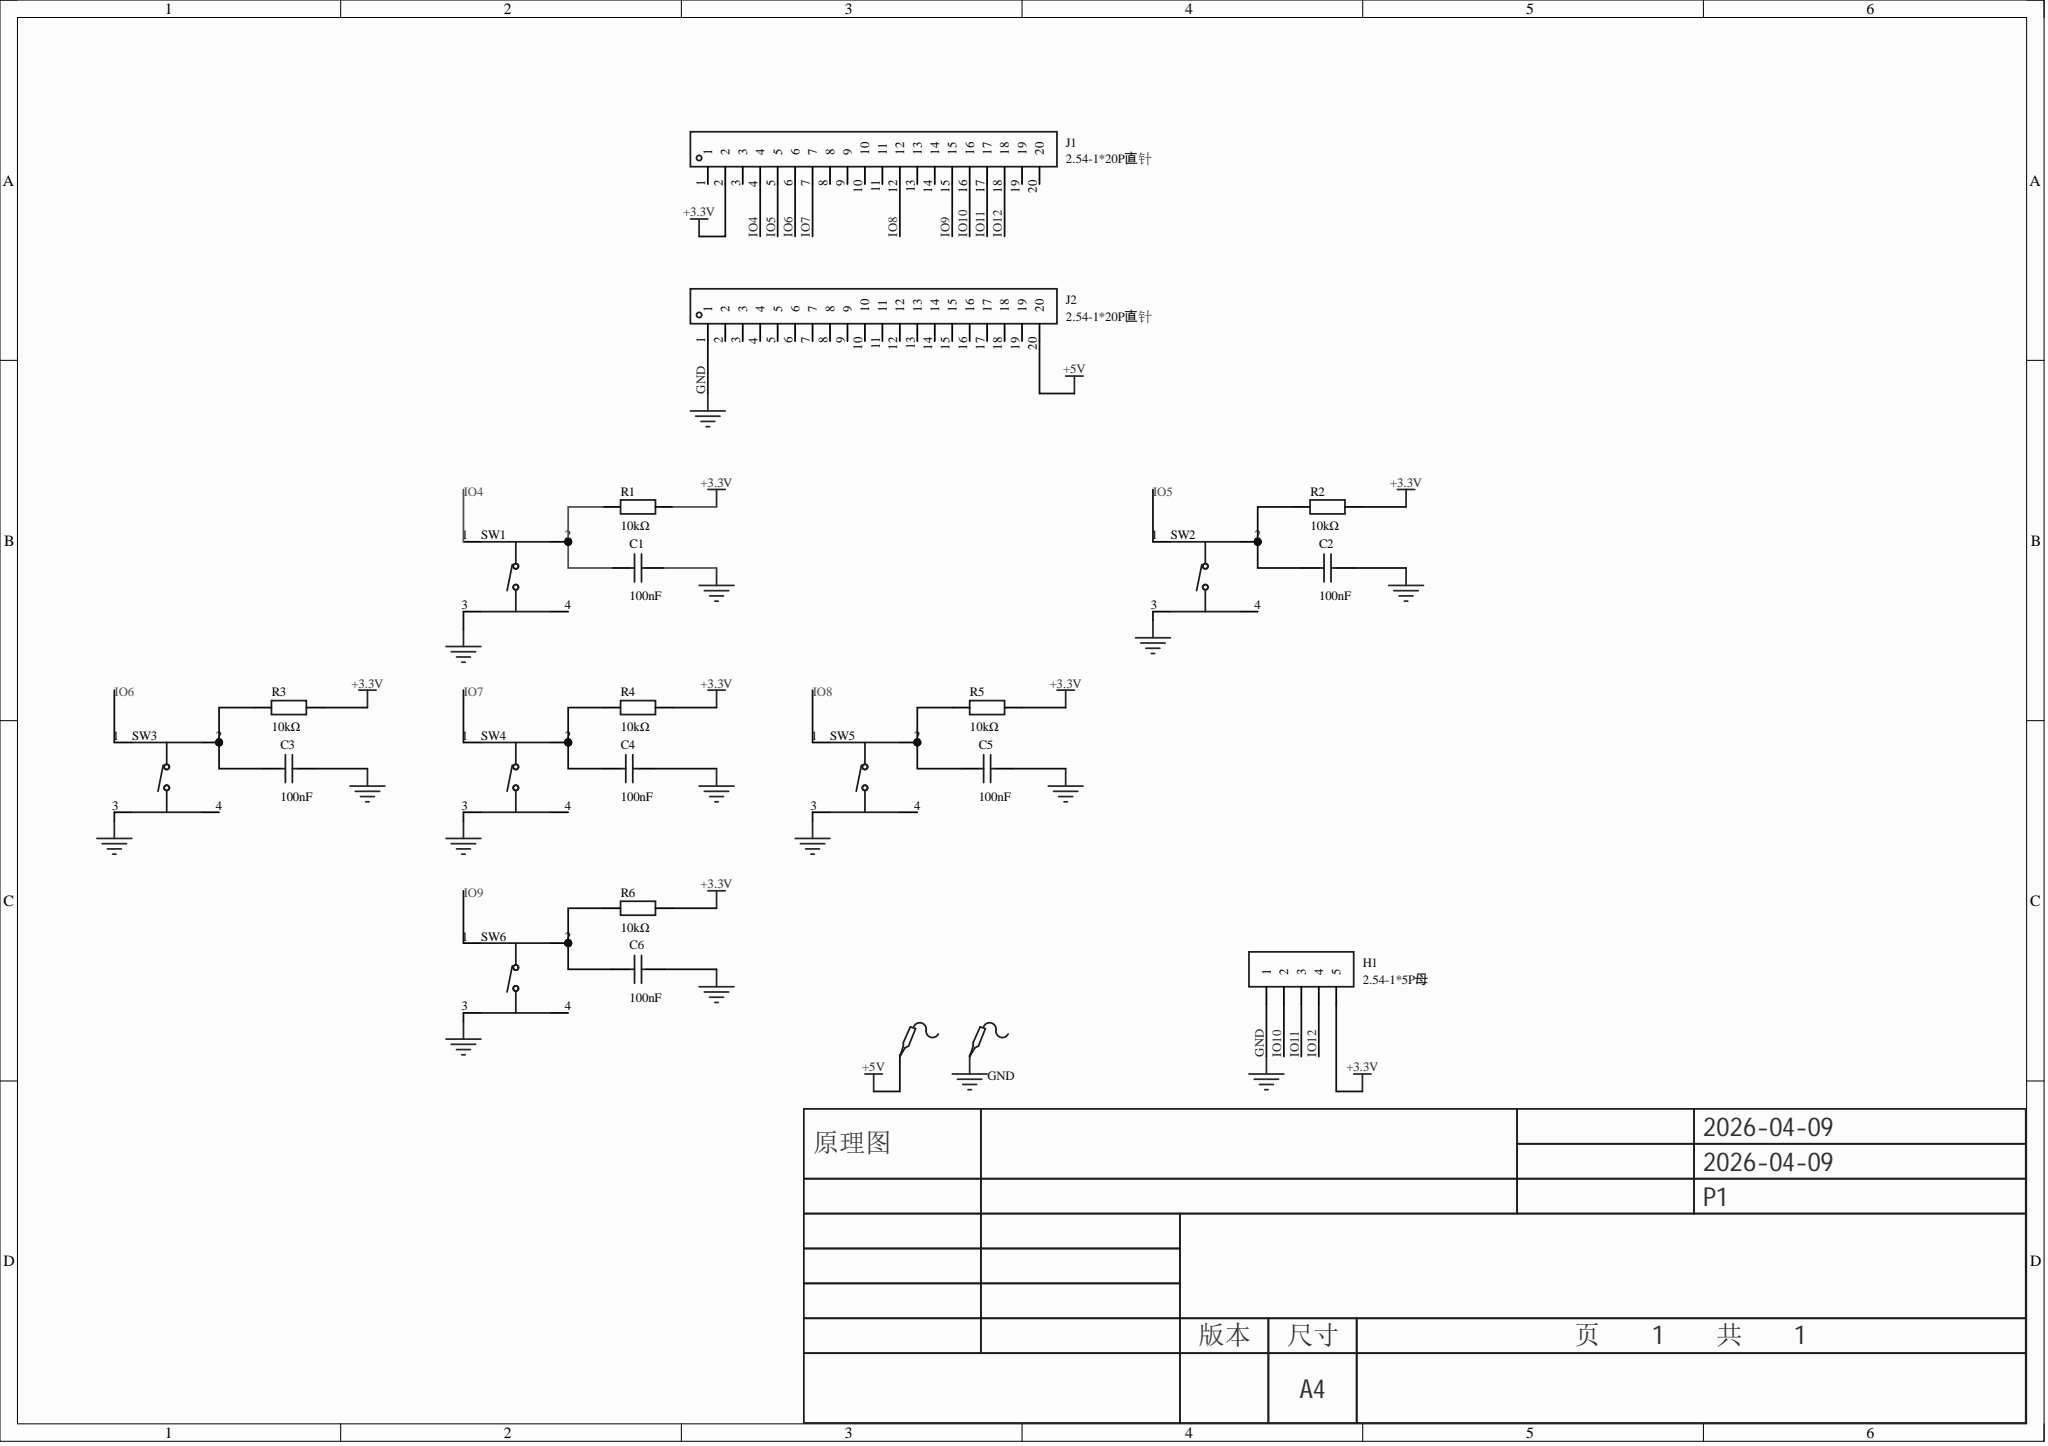Circuit board | Altium Designer | 23 parts | 18 nets
Bill of materials:
Comment,Description,Designator,Footprint,LibRef,Quantity
"","Test-Point","5V, GND","Test-Point-0.5mm","Test-Point","2"
"100nF","容值:100nF;精度:±10%;额定电压:100V;材质(温度系数):X7R;","C1, C2, C3, C4, C5, C6","C0805","CC0805KKX7R0BB104","6"
"2.54-1*5P母","间距:2.54mm;总孔位数:5;排数:1;插孔结构:1x5P;行距:-;安装类型:直插;塑高:-;触头材质:-;触头镀层:-;","H1","HDR-TH_5P-P2.54-V-F","2.54-1*5P母","1"
"2.54-1*20P直针","间距:2.54mm;总PIN位数:20;排数:1;插针结构:1x20P;行距:-;安装类型:直插;圆针/方针:方针;额定电流:3A;额定电压:-;配合针长度:-;塑高:-;端接针长度:-;触头材质:黄铜;触头镀层:-;工作温度范围:-40℃~+105℃;颜色:黑色;","J1, J2","HDR-TH_20P-P2.54-V-M-1","2.54-1*20P直针","2"
"10kΩ","","R1, R2, R3, R4, R5, R6","R0805","CR0805J80103G","6"
"TC-1103-C-K","","SW1, SW2, SW3, SW4, SW5, SW6","KEY-TH_4P-L12.0-W12.0-P5.00-LS12.5","TC-1103-C-K","6"
Netlist (Protel format):
[
5V
Test-Point-0.5mm




]
[
C1
C0805
100nF



]
[
C2
C0805
100nF



]
[
C3
C0805
100nF



]
[
C4
C0805
100nF



]
[
C5
C0805
100nF



]
[
C6
C0805
100nF



]
[
GND
Test-Point-0.5mm




]
[
H1
HDR-TH_5P-P2.54-V-F
2.54-1*5P母



]
[
J1
HDR-TH_20P-P2.54-V-M-1
2.54-1*20P直针



]
[
J2
HDR-TH_20P-P2.54-V-M-1
2.54-1*20P直针



]
[
R1
R0805
10kΩ



]
[
R2
R0805
10kΩ



]
[
R3
R0805
10kΩ



]
[
R4
R0805
10kΩ



]
[
R5
R0805
10kΩ



]
[
R6
R0805
10kΩ



]
[
SW1
KEY-TH_4P-L12.0-W12.0-P5.00-LS12.5
TC-1103-C-K



]
[
SW2
KEY-TH_4P-L12.0-W12.0-P5.00-LS12.5
TC-1103-C-K



]
[
SW3
KEY-TH_4P-L12.0-W12.0-P5.00-LS12.5
TC-1103-C-K



]
[
SW4
KEY-TH_4P-L12.0-W12.0-P5.00-LS12.5
TC-1103-C-K



]
[
SW5
KEY-TH_4P-L12.0-W12.0-P5.00-LS12.5
TC-1103-C-K



]
[
SW6
KEY-TH_4P-L12.0-W12.0-P5.00-LS12.5
TC-1103-C-K



]
(
NetC6_1
C6-1
R6-1
SW6-2
)
(
NetC5_1
C5-1
R5-1
SW5-2
)
(
NetC4_1
C4-1
R4-1
SW4-2
)
(
NetC3_1
C3-1
R3-1
SW3-2
)
(
NetC2_1
C2-1
R2-1
SW2-2
)
(
NetC1_1
C1-1
R1-1
SW1-2
)
(
IO12
H1-4
J1-18
)
(
IO11
H1-3
J1-17
)
(
IO10
H1-2
J1-16
)
(
IO9
J1-15
SW6-1
)
(
IO8
J1-12
SW5-1
)
(
IO7
J1-7
SW4-1
)
(
IO6
J1-6
SW3-1
)
(
IO5
J1-5
SW2-1
)
(
IO4
J1-4
SW1-1
)
(
GND
C1-2
C2-2
C3-2
C4-2
C5-2
C6-2
GND-1
H1-1
J2-1
SW1-3
SW2-3
SW3-3
SW4-3
SW5-3
SW6-3
)
(
+5V
5V-1
J2-20
)
(
+3.3V
H1-5
J1-2
R1-2
R2-2
R3-2
R4-2
R5-2
R6-2
)